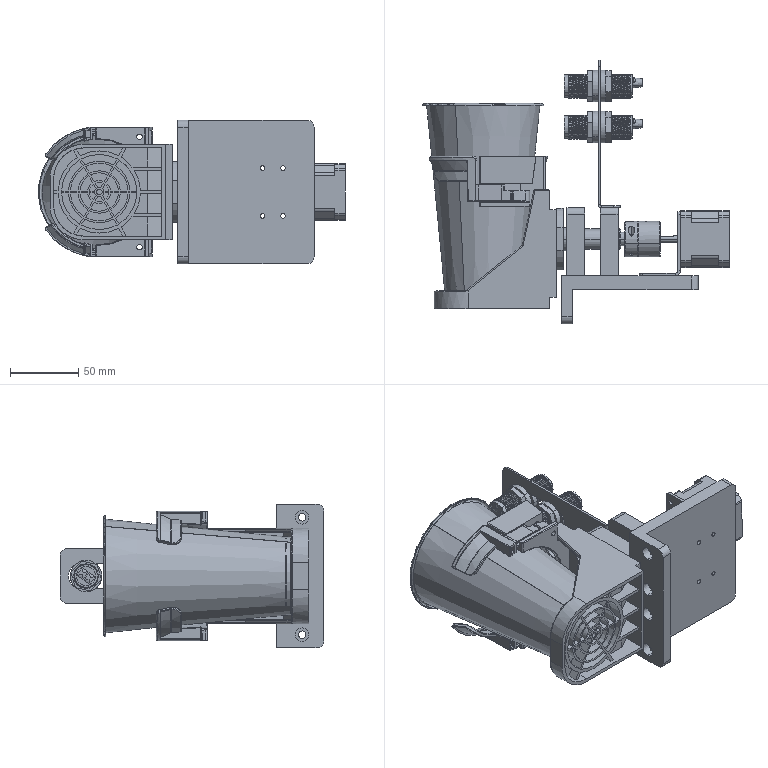Part | SolidWorks | features ReferencePattern 3, AEMSimFeature 1, InContextFeatHolder 1, LocalLPattern 1 | 24 solids | 1876 faces | box 224.692 x 193 x 105 mm | volume 423865 mm3 | cylinder 810 | plane 626 | cone 181 | torus 129 | spline 114 | sphere 16 | commonest cylinder face diameters 17.6 x168 1 x111 17 x80 4 x27 3.3 x24 10 x24